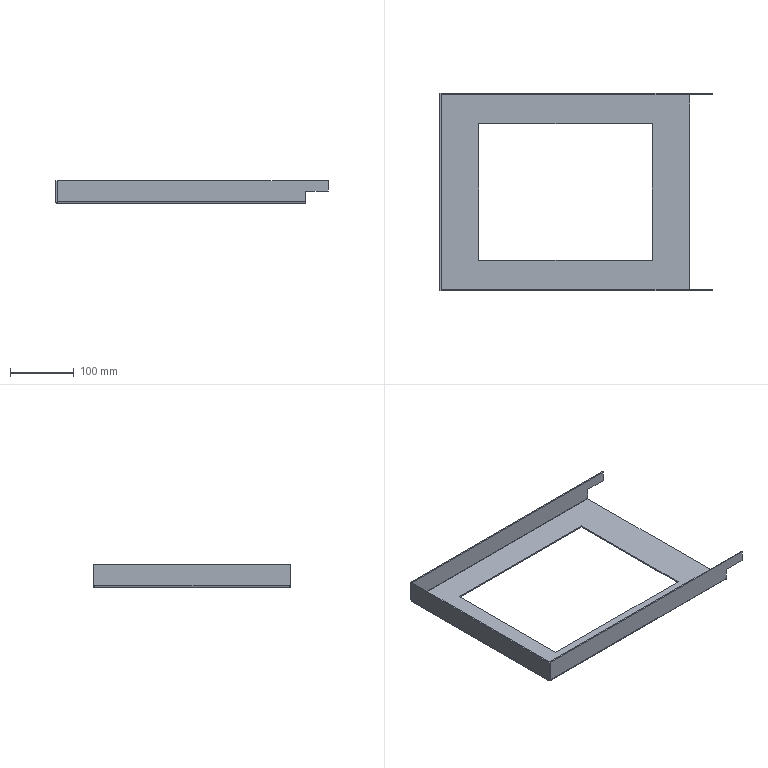Part | SolidWorks | features BaseBody 1 | 1 solid | 40 faces | box 428 x 310 x 36 mm | volume 201770 mm3 | plane 34 | cylinder 6 | commonest cylinder face diameters 1 x3 5 x3
STEP:
#1=CARTESIAN_POINT('',(196.5,-155.,17.5));
#2=VERTEX_POINT('',#1);
#3=CARTESIAN_POINT('',(231.5,-155.,17.5));
#4=VERTEX_POINT('',#3);
#5=CARTESIAN_POINT('',(196.5,-155.,17.5));
#6=DIRECTION('',(1.,0.,0.));
#7=VECTOR('',#6,1000.);
#8=LINE('',#5,#7);
#9=EDGE_CURVE('',#2,#4,#8,.T.);
#10=ORIENTED_EDGE('',*,*,#9,.F.);
#11=CARTESIAN_POINT('',(196.5,-153.,17.5));
#12=VERTEX_POINT('',#11);
#13=CARTESIAN_POINT('',(196.5,-153.,17.5));
#14=DIRECTION('',(0.,-1.,0.));
#15=VECTOR('',#14,1000.);
#16=LINE('',#13,#15);
#17=EDGE_CURVE('',#12,#2,#16,.T.);
#18=ORIENTED_EDGE('',*,*,#17,.F.);
#19=CARTESIAN_POINT('',(231.5,-153.,17.5));
#20=VERTEX_POINT('',#19);
#21=CARTESIAN_POINT('',(196.5,-153.,17.5));
#22=DIRECTION('',(1.,0.,0.));
#23=VECTOR('',#22,1000.);
#24=LINE('',#21,#23);
#25=EDGE_CURVE('',#12,#20,#24,.T.);
#26=ORIENTED_EDGE('',*,*,#25,.T.);
#27=CARTESIAN_POINT('',(231.5,-153.,17.5));
#28=DIRECTION('',(0.,-1.,0.));
#29=VECTOR('',#28,1000.);
#30=LINE('',#27,#29);
#31=EDGE_CURVE('',#20,#4,#30,.T.);
#32=ORIENTED_EDGE('',*,*,#31,.T.);
#33=EDGE_LOOP('',(#10,#18,#26,#32));
#34=FACE_OUTER_BOUND('',#33,.T.);
#35=CARTESIAN_POINT('',(196.5,-153.,17.5));
#36=DIRECTION('',(0.,0.,-1.));
#37=DIRECTION('',(-1.,0.,0.));
#38=AXIS2_PLACEMENT_3D('',#35,#36,#37);
#39=PLANE('',#38);
#40=ADVANCED_FACE('',(#34),#39,.T.);
#41=CARTESIAN_POINT('',(231.5,-155.,34.));
#42=VERTEX_POINT('',#41);
#43=CARTESIAN_POINT('',(231.5,-155.,34.));
#44=DIRECTION('',(0.,0.,1.));
#45=VECTOR('',#44,1000.);
#46=LINE('',#43,#45);
#47=EDGE_CURVE('',#4,#42,#46,.T.);
#48=ORIENTED_EDGE('',*,*,#47,.F.);
#49=ORIENTED_EDGE('',*,*,#31,.F.);
#50=CARTESIAN_POINT('',(231.5,-153.,34.));
#51=VERTEX_POINT('',#50);
#52=CARTESIAN_POINT('',(231.5,-153.,34.));
#53=DIRECTION('',(0.,0.,1.));
#54=VECTOR('',#53,1000.);
#55=LINE('',#52,#54);
#56=EDGE_CURVE('',#20,#51,#55,.T.);
#57=ORIENTED_EDGE('',*,*,#56,.T.);
#58=CARTESIAN_POINT('',(231.5,-153.,34.));
#59=DIRECTION('',(0.,-1.,0.));
#60=VECTOR('',#59,1000.);
#61=LINE('',#58,#60);
#62=EDGE_CURVE('',#51,#42,#61,.T.);
#63=ORIENTED_EDGE('',*,*,#62,.T.);
#64=EDGE_LOOP('',(#48,#49,#57,#63));
#65=FACE_OUTER_BOUND('',#64,.T.);
#66=CARTESIAN_POINT('',(231.5,-153.,34.));
#67=DIRECTION('',(1.,0.,0.));
#68=DIRECTION('',(0.,1.,0.));
#69=AXIS2_PLACEMENT_3D('',#66,#67,#68);
#70=PLANE('',#69);
#71=ADVANCED_FACE('',(#65),#70,.T.);
#72=CARTESIAN_POINT('',(137.,-107.5,-2.));
#73=VERTEX_POINT('',#72);
#74=CARTESIAN_POINT('',(-135.,-107.5,-2.));
#75=VERTEX_POINT('',#74);
#76=CARTESIAN_POINT('',(-135.,-107.5,-2.));
#77=DIRECTION('',(-1.,0.,0.));
#78=VECTOR('',#77,1000.);
#79=LINE('',#76,#78);
#80=EDGE_CURVE('',#73,#75,#79,.T.);
#81=ORIENTED_EDGE('',*,*,#80,.T.);
#82=CARTESIAN_POINT('',(-135.,-107.5,0.));
#83=VERTEX_POINT('',#82);
#84=CARTESIAN_POINT('',(-135.,-107.5,0.));
#85=DIRECTION('',(0.,0.,-1.));
#86=VECTOR('',#85,1000.);
#87=LINE('',#84,#86);
#88=EDGE_CURVE('',#83,#75,#87,.T.);
#89=ORIENTED_EDGE('',*,*,#88,.F.);
#90=CARTESIAN_POINT('',(137.,-107.5,0.));
#91=VERTEX_POINT('',#90);
#92=CARTESIAN_POINT('',(-135.,-107.5,0.));
#93=DIRECTION('',(-1.,0.,0.));
#94=VECTOR('',#93,1000.);
#95=LINE('',#92,#94);
#96=EDGE_CURVE('',#91,#83,#95,.T.);
#97=ORIENTED_EDGE('',*,*,#96,.F.);
#98=CARTESIAN_POINT('',(137.,-107.5,0.));
#99=DIRECTION('',(0.,0.,-1.));
#100=VECTOR('',#99,1000.);
#101=LINE('',#98,#100);
#102=EDGE_CURVE('',#91,#73,#101,.T.);
#103=ORIENTED_EDGE('',*,*,#102,.T.);
#104=EDGE_LOOP('',(#81,#89,#97,#103));
#105=FACE_OUTER_BOUND('',#104,.T.);
#106=CARTESIAN_POINT('',(-135.,-107.5,0.));
#107=DIRECTION('',(0.,-1.,0.));
#108=DIRECTION('',(-1.,0.,0.));
#109=AXIS2_PLACEMENT_3D('',#106,#107,#108);
#110=PLANE('',#109);
#111=ADVANCED_FACE('',(#105),#110,.F.);
#112=CARTESIAN_POINT('',(-135.,107.5,-2.));
#113=VERTEX_POINT('',#112);
#114=CARTESIAN_POINT('',(-135.,107.5,-2.));
#115=DIRECTION('',(0.,1.,0.));
#116=VECTOR('',#115,1000.);
#117=LINE('',#114,#116);
#118=EDGE_CURVE('',#75,#113,#117,.T.);
#119=ORIENTED_EDGE('',*,*,#118,.T.);
#120=CARTESIAN_POINT('',(-135.,107.5,0.));
#121=VERTEX_POINT('',#120);
#122=CARTESIAN_POINT('',(-135.,107.5,0.));
#123=DIRECTION('',(0.,0.,-1.));
#124=VECTOR('',#123,1000.);
#125=LINE('',#122,#124);
#126=EDGE_CURVE('',#121,#113,#125,.T.);
#127=ORIENTED_EDGE('',*,*,#126,.F.);
#128=CARTESIAN_POINT('',(-135.,107.5,0.));
#129=DIRECTION('',(0.,1.,0.));
#130=VECTOR('',#129,1000.);
#131=LINE('',#128,#130);
#132=EDGE_CURVE('',#83,#121,#131,.T.);
#133=ORIENTED_EDGE('',*,*,#132,.F.);
#134=ORIENTED_EDGE('',*,*,#88,.T.);
#135=EDGE_LOOP('',(#119,#127,#133,#134));
#136=FACE_OUTER_BOUND('',#135,.T.);
#137=CARTESIAN_POINT('',(-135.,107.5,0.));
#138=DIRECTION('',(-1.,0.,0.));
#139=DIRECTION('',(0.,0.,1.));
#140=AXIS2_PLACEMENT_3D('',#137,#138,#139);
#141=PLANE('',#140);
#142=ADVANCED_FACE('',(#136),#141,.F.);
#143=CARTESIAN_POINT('',(137.,107.5,-2.));
#144=VERTEX_POINT('',#143);
#145=CARTESIAN_POINT('',(-135.,107.5,-2.));
#146=DIRECTION('',(1.,0.,0.));
#147=VECTOR('',#146,1000.);
#148=LINE('',#145,#147);
#149=EDGE_CURVE('',#113,#144,#148,.T.);
#150=ORIENTED_EDGE('',*,*,#149,.T.);
#151=CARTESIAN_POINT('',(137.,107.5,0.));
#152=VERTEX_POINT('',#151);
#153=CARTESIAN_POINT('',(137.,107.5,0.));
#154=DIRECTION('',(0.,0.,-1.));
#155=VECTOR('',#154,1000.);
#156=LINE('',#153,#155);
#157=EDGE_CURVE('',#152,#144,#156,.T.);
#158=ORIENTED_EDGE('',*,*,#157,.F.);
#159=CARTESIAN_POINT('',(-135.,107.5,0.));
#160=DIRECTION('',(1.,0.,0.));
#161=VECTOR('',#160,1000.);
#162=LINE('',#159,#161);
#163=EDGE_CURVE('',#121,#152,#162,.T.);
#164=ORIENTED_EDGE('',*,*,#163,.F.);
#165=ORIENTED_EDGE('',*,*,#126,.T.);
#166=EDGE_LOOP('',(#150,#158,#164,#165));
#167=FACE_OUTER_BOUND('',#166,.T.);
#168=CARTESIAN_POINT('',(-135.,107.5,0.));
#169=DIRECTION('',(0.,1.,0.));
#170=DIRECTION('',(1.,0.,0.));
#171=AXIS2_PLACEMENT_3D('',#168,#169,#170);
#172=PLANE('',#171);
#173=ADVANCED_FACE('',(#167),#172,.F.);
#174=CARTESIAN_POINT('',(137.,107.5,-2.));
#175=DIRECTION('',(0.,-1.,0.));
#176=VECTOR('',#175,1000.);
#177=LINE('',#174,#176);
#178=EDGE_CURVE('',#144,#73,#177,.T.);
#179=ORIENTED_EDGE('',*,*,#178,.T.);
#180=ORIENTED_EDGE('',*,*,#102,.F.);
#181=CARTESIAN_POINT('',(137.,107.5,0.));
#182=DIRECTION('',(0.,-1.,0.));
#183=VECTOR('',#182,1000.);
#184=LINE('',#181,#183);
#185=EDGE_CURVE('',#152,#91,#184,.T.);
#186=ORIENTED_EDGE('',*,*,#185,.F.);
#187=ORIENTED_EDGE('',*,*,#157,.T.);
#188=EDGE_LOOP('',(#179,#180,#186,#187));
#189=FACE_OUTER_BOUND('',#188,.T.);
#190=CARTESIAN_POINT('',(137.,107.5,0.));
#191=DIRECTION('',(1.,0.,0.));
#192=DIRECTION('',(0.,-1.,0.));
#193=AXIS2_PLACEMENT_3D('',#190,#191,#192);
#194=PLANE('',#193);
#195=ADVANCED_FACE('',(#189),#194,.F.);
#196=CARTESIAN_POINT('',(231.5,155.,34.));
#197=VERTEX_POINT('',#196);
#198=CARTESIAN_POINT('',(231.5,155.,17.5));
#199=VERTEX_POINT('',#198);
#200=CARTESIAN_POINT('',(231.5,155.,34.));
#201=DIRECTION('',(0.,0.,-1.));
#202=VECTOR('',#201,1000.);
#203=LINE('',#200,#202);
#204=EDGE_CURVE('',#197,#199,#203,.T.);
#205=ORIENTED_EDGE('',*,*,#204,.F.);
#206=CARTESIAN_POINT('',(231.5,153.,34.));
#207=VERTEX_POINT('',#206);
#208=CARTESIAN_POINT('',(231.5,153.,34.));
#209=DIRECTION('',(0.,1.,0.));
#210=VECTOR('',#209,1000.);
#211=LINE('',#208,#210);
#212=EDGE_CURVE('',#207,#197,#211,.T.);
#213=ORIENTED_EDGE('',*,*,#212,.F.);
#214=CARTESIAN_POINT('',(231.5,153.,17.5));
#215=VERTEX_POINT('',#214);
#216=CARTESIAN_POINT('',(231.5,153.,34.));
#217=DIRECTION('',(0.,0.,-1.));
#218=VECTOR('',#217,1000.);
#219=LINE('',#216,#218);
#220=EDGE_CURVE('',#207,#215,#219,.T.);
#221=ORIENTED_EDGE('',*,*,#220,.T.);
#222=CARTESIAN_POINT('',(231.5,153.,17.5));
#223=DIRECTION('',(0.,1.,0.));
#224=VECTOR('',#223,1000.);
#225=LINE('',#222,#224);
#226=EDGE_CURVE('',#215,#199,#225,.T.);
#227=ORIENTED_EDGE('',*,*,#226,.T.);
#228=EDGE_LOOP('',(#205,#213,#221,#227));
#229=FACE_OUTER_BOUND('',#228,.T.);
#230=CARTESIAN_POINT('',(231.5,153.,34.));
#231=DIRECTION('',(1.,0.,0.));
#232=DIRECTION('',(0.,1.,0.));
#233=AXIS2_PLACEMENT_3D('',#230,#231,#232);
#234=PLANE('',#233);
#235=ADVANCED_FACE('',(#229),#234,.T.);
#236=CARTESIAN_POINT('',(196.5,155.,17.5));
#237=VERTEX_POINT('',#236);
#238=CARTESIAN_POINT('',(196.5,155.,17.5));
#239=DIRECTION('',(-1.,0.,0.));
#240=VECTOR('',#239,1000.);
#241=LINE('',#238,#240);
#242=EDGE_CURVE('',#199,#237,#241,.T.);
#243=ORIENTED_EDGE('',*,*,#242,.F.);
#244=ORIENTED_EDGE('',*,*,#226,.F.);
#245=CARTESIAN_POINT('',(196.5,153.,17.5));
#246=VERTEX_POINT('',#245);
#247=CARTESIAN_POINT('',(196.5,153.,17.5));
#248=DIRECTION('',(-1.,0.,0.));
#249=VECTOR('',#248,1000.);
#250=LINE('',#247,#249);
#251=EDGE_CURVE('',#215,#246,#250,.T.);
#252=ORIENTED_EDGE('',*,*,#251,.T.);
#253=CARTESIAN_POINT('',(196.5,153.,17.5));
#254=DIRECTION('',(0.,1.,0.));
#255=VECTOR('',#254,1000.);
#256=LINE('',#253,#255);
#257=EDGE_CURVE('',#246,#237,#256,.T.);
#258=ORIENTED_EDGE('',*,*,#257,.T.);
#259=EDGE_LOOP('',(#243,#244,#252,#258));
#260=FACE_OUTER_BOUND('',#259,.T.);
#261=CARTESIAN_POINT('',(196.5,153.,17.5));
#262=DIRECTION('',(0.,0.,-1.));
#263=DIRECTION('',(0.,-1.,0.));
#264=AXIS2_PLACEMENT_3D('',#261,#262,#263);
#265=PLANE('',#264);
#266=ADVANCED_FACE('',(#260),#265,.T.);
#267=CARTESIAN_POINT('',(-194.,-153.,34.));
#268=VERTEX_POINT('',#267);
#269=CARTESIAN_POINT('',(-194.,-153.,34.));
#270=DIRECTION('',(-1.,0.,0.));
#271=VECTOR('',#270,1000.);
#272=LINE('',#269,#271);
#273=EDGE_CURVE('',#51,#268,#272,.T.);
#274=ORIENTED_EDGE('',*,*,#273,.T.);
#275=CARTESIAN_POINT('',(-194.,-155.,34.));
#276=VERTEX_POINT('',#275);
#277=CARTESIAN_POINT('',(-194.,-155.,34.));
#278=DIRECTION('',(0.,1.,0.));
#279=VECTOR('',#278,1000.);
#280=LINE('',#277,#279);
#281=EDGE_CURVE('',#276,#268,#280,.T.);
#282=ORIENTED_EDGE('',*,*,#281,.F.);
#283=CARTESIAN_POINT('',(0.,-155.,34.));
#284=DIRECTION('',(-1.,0.,0.));
#285=VECTOR('',#284,1000.);
#286=LINE('',#283,#285);
#287=EDGE_CURVE('',#42,#276,#286,.T.);
#288=ORIENTED_EDGE('',*,*,#287,.F.);
#289=ORIENTED_EDGE('',*,*,#62,.F.);
#290=EDGE_LOOP('',(#274,#282,#288,#289));
#291=FACE_OUTER_BOUND('',#290,.T.);
#292=CARTESIAN_POINT('',(-194.,-155.,34.));
#293=DIRECTION('',(0.,0.,-1.));
#294=DIRECTION('',(-1.,0.,0.));
#295=AXIS2_PLACEMENT_3D('',#292,#293,#294);
#296=PLANE('',#295);
#297=ADVANCED_FACE('',(#291),#296,.F.);
#298=CARTESIAN_POINT('',(196.5,-153.,0.5));
#299=VERTEX_POINT('',#298);
#300=CARTESIAN_POINT('',(196.5,-153.,34.));
#301=DIRECTION('',(0.,0.,1.));
#302=VECTOR('',#301,1000.);
#303=LINE('',#300,#302);
#304=EDGE_CURVE('',#299,#12,#303,.T.);
#305=ORIENTED_EDGE('',*,*,#304,.F.);
#306=CARTESIAN_POINT('',(-194.,-153.,0.5));
#307=VERTEX_POINT('',#306);
#308=CARTESIAN_POINT('',(-194.,-153.,0.5));
#309=DIRECTION('',(1.,0.,0.));
#310=VECTOR('',#309,1000.);
#311=LINE('',#308,#310);
#312=EDGE_CURVE('',#307,#299,#311,.T.);
#313=ORIENTED_EDGE('',*,*,#312,.F.);
#314=CARTESIAN_POINT('',(-194.,-153.,0.));
#315=DIRECTION('',(0.,0.,-1.));
#316=VECTOR('',#315,1000.);
#317=LINE('',#314,#316);
#318=EDGE_CURVE('',#268,#307,#317,.T.);
#319=ORIENTED_EDGE('',*,*,#318,.F.);
#320=ORIENTED_EDGE('',*,*,#273,.F.);
#321=ORIENTED_EDGE('',*,*,#56,.F.);
#322=ORIENTED_EDGE('',*,*,#25,.F.);
#323=EDGE_LOOP('',(#305,#313,#319,#320,#321,#322));
#324=FACE_OUTER_BOUND('',#323,.T.);
#325=CARTESIAN_POINT('',(0.,-153.,0.));
#326=DIRECTION('',(0.,1.,0.));
#327=DIRECTION('',(0.,0.,-1.));
#328=AXIS2_PLACEMENT_3D('',#325,#326,#327);
#329=PLANE('',#328);
#330=ADVANCED_FACE('',(#324),#329,.T.);
#331=CARTESIAN_POINT('',(196.5,-155.,0.5));
#332=VERTEX_POINT('',#331);
#333=CARTESIAN_POINT('',(-194.,-155.,0.5));
#334=VERTEX_POINT('',#333);
#335=CARTESIAN_POINT('',(-194.,-155.,0.5));
#336=DIRECTION('',(-1.,0.,0.));
#337=VECTOR('',#336,1000.);
#338=LINE('',#335,#337);
#339=EDGE_CURVE('',#332,#334,#338,.T.);
#340=ORIENTED_EDGE('',*,*,#339,.F.);
#341=CARTESIAN_POINT('',(196.5,-155.,0.));
#342=DIRECTION('',(0.,0.,1.));
#343=VECTOR('',#342,1000.);
#344=LINE('',#341,#343);
#345=EDGE_CURVE('',#332,#2,#344,.T.);
#346=ORIENTED_EDGE('',*,*,#345,.T.);
#347=ORIENTED_EDGE('',*,*,#9,.T.);
#348=ORIENTED_EDGE('',*,*,#47,.T.);
#349=ORIENTED_EDGE('',*,*,#287,.T.);
#350=CARTESIAN_POINT('',(-194.,-155.,0.));
#351=DIRECTION('',(0.,0.,-1.));
#352=VECTOR('',#351,1000.);
#353=LINE('',#350,#352);
#354=EDGE_CURVE('',#276,#334,#353,.T.);
#355=ORIENTED_EDGE('',*,*,#354,.T.);
#356=EDGE_LOOP('',(#340,#346,#347,#348,#349,#355));
#357=FACE_OUTER_BOUND('',#356,.T.);
#358=CARTESIAN_POINT('',(0.,-155.,0.));
#359=DIRECTION('',(0.,1.,0.));
#360=DIRECTION('',(0.,0.,-1.));
#361=AXIS2_PLACEMENT_3D('',#358,#359,#360);
#362=PLANE('',#361);
#363=ADVANCED_FACE('',(#357),#362,.F.);
#364=CARTESIAN_POINT('',(-194.,-155.,0.5));
#365=DIRECTION('',(0.,-1.,0.));
#366=VECTOR('',#365,1000.);
#367=LINE('',#364,#366);
#368=EDGE_CURVE('',#307,#334,#367,.T.);
#369=ORIENTED_EDGE('',*,*,#368,.T.);
#370=ORIENTED_EDGE('',*,*,#354,.F.);
#371=ORIENTED_EDGE('',*,*,#281,.T.);
#372=ORIENTED_EDGE('',*,*,#318,.T.);
#373=EDGE_LOOP('',(#369,#370,#371,#372));
#374=FACE_OUTER_BOUND('',#373,.T.);
#375=CARTESIAN_POINT('',(-194.,-155.,0.));
#376=DIRECTION('',(1.,0.,0.));
#377=DIRECTION('',(0.,1.,0.));
#378=AXIS2_PLACEMENT_3D('',#375,#376,#377);
#379=PLANE('',#378);
#380=ADVANCED_FACE('',(#374),#379,.F.);
#381=ORIENTED_EDGE('',*,*,#304,.T.);
#382=ORIENTED_EDGE('',*,*,#17,.T.);
#383=ORIENTED_EDGE('',*,*,#345,.F.);
#384=CARTESIAN_POINT('',(196.5,-153.,0.5));
#385=DIRECTION('',(0.,-1.,0.));
#386=VECTOR('',#385,1000.);
#387=LINE('',#384,#386);
#388=EDGE_CURVE('',#299,#332,#387,.T.);
#389=ORIENTED_EDGE('',*,*,#388,.F.);
#390=EDGE_LOOP('',(#381,#382,#383,#389));
#391=FACE_OUTER_BOUND('',#390,.T.);
#392=CARTESIAN_POINT('',(196.5,-155.,34.));
#393=DIRECTION('',(-1.,0.,0.));
#394=DIRECTION('',(0.,1.,0.));
#395=AXIS2_PLACEMENT_3D('',#392,#393,#394);
#396=PLANE('',#395);
#397=ADVANCED_FACE('',(#391),#396,.F.);
#398=CARTESIAN_POINT('',(196.5,-152.5,0.));
#399=VERTEX_POINT('',#398);
#400=CARTESIAN_POINT('',(-194.,-152.5,0.));
#401=VERTEX_POINT('',#400);
#402=CARTESIAN_POINT('',(196.5,-152.5,0.));
#403=DIRECTION('',(-1.,0.,0.));
#404=VECTOR('',#403,1000.);
#405=LINE('',#402,#404);
#406=EDGE_CURVE('',#399,#401,#405,.T.);
#407=ORIENTED_EDGE('',*,*,#406,.T.);
#408=CARTESIAN_POINT('',(-194.,-152.5,0.5));
#409=DIRECTION('',(-1.,0.,0.));
#410=DIRECTION('',(0.,0.,-1.));
#411=AXIS2_PLACEMENT_3D('',#408,#409,#410);
#412=CIRCLE('',#411,0.5);
#413=EDGE_CURVE('',#401,#307,#412,.T.);
#414=ORIENTED_EDGE('',*,*,#413,.T.);
#415=ORIENTED_EDGE('',*,*,#312,.T.);
#416=CARTESIAN_POINT('',(196.5,-152.5,0.5));
#417=DIRECTION('',(1.,0.,0.));
#418=DIRECTION('',(0.,0.,-1.));
#419=AXIS2_PLACEMENT_3D('',#416,#417,#418);
#420=CIRCLE('',#419,0.5);
#421=EDGE_CURVE('',#299,#399,#420,.T.);
#422=ORIENTED_EDGE('',*,*,#421,.T.);
#423=EDGE_LOOP('',(#407,#414,#415,#422));
#424=FACE_OUTER_BOUND('',#423,.T.);
#425=CARTESIAN_POINT('',(196.5,-152.5,0.5));
#426=DIRECTION('',(1.,0.,0.));
#427=DIRECTION('',(0.,-1.,0.));
#428=AXIS2_PLACEMENT_3D('',#425,#426,#427);
#429=CYLINDRICAL_SURFACE('',#428,0.5);
#430=ADVANCED_FACE('',(#424),#429,.F.);
#431=CARTESIAN_POINT('',(196.5,-152.5,-2.));
#432=VERTEX_POINT('',#431);
#433=CARTESIAN_POINT('',(-194.,-152.5,-2.));
#434=VERTEX_POINT('',#433);
#435=CARTESIAN_POINT('',(196.5,-152.5,-2.));
#436=DIRECTION('',(-1.,0.,0.));
#437=VECTOR('',#436,1000.);
#438=LINE('',#435,#437);
#439=EDGE_CURVE('',#432,#434,#438,.T.);
#440=ORIENTED_EDGE('',*,*,#439,.F.);
#441=CARTESIAN_POINT('',(196.5,-152.5,0.5));
#442=DIRECTION('',(1.,0.,0.));
#443=DIRECTION('',(0.,0.,-1.));
#444=AXIS2_PLACEMENT_3D('',#441,#442,#443);
#445=CIRCLE('',#444,2.5);
#446=EDGE_CURVE('',#332,#432,#445,.T.);
#447=ORIENTED_EDGE('',*,*,#446,.F.);
#448=ORIENTED_EDGE('',*,*,#339,.T.);
#449=CARTESIAN_POINT('',(-194.,-152.5,0.5));
#450=DIRECTION('',(-1.,0.,0.));
#451=DIRECTION('',(0.,0.,-1.));
#452=AXIS2_PLACEMENT_3D('',#449,#450,#451);
#453=CIRCLE('',#452,2.5);
#454=EDGE_CURVE('',#434,#334,#453,.T.);
#455=ORIENTED_EDGE('',*,*,#454,.F.);
#456=EDGE_LOOP('',(#440,#447,#448,#455));
#457=FACE_OUTER_BOUND('',#456,.T.);
#458=CARTESIAN_POINT('',(196.5,-152.5,0.5));
#459=DIRECTION('',(1.,0.,0.));
#460=DIRECTION('',(0.,-1.,0.));
#461=AXIS2_PLACEMENT_3D('',#458,#459,#460);
#462=CYLINDRICAL_SURFACE('',#461,2.5);
#463=ADVANCED_FACE('',(#457),#462,.T.);
#464=ORIENTED_EDGE('',*,*,#421,.F.);
#465=ORIENTED_EDGE('',*,*,#388,.T.);
#466=ORIENTED_EDGE('',*,*,#446,.T.);
#467=CARTESIAN_POINT('',(196.5,-152.5,0.));
#468=DIRECTION('',(0.,0.,-1.));
#469=VECTOR('',#468,1000.);
#470=LINE('',#467,#469);
#471=EDGE_CURVE('',#399,#432,#470,.T.);
#472=ORIENTED_EDGE('',*,*,#471,.F.);
#473=EDGE_LOOP('',(#464,#465,#466,#472));
#474=FACE_OUTER_BOUND('',#473,.T.);
#475=CARTESIAN_POINT('',(196.5,-152.5,0.5));
#476=DIRECTION('',(-1.,0.,0.));
#477=DIRECTION('',(0.,1.,0.));
#478=AXIS2_PLACEMENT_3D('',#475,#476,#477);
#479=PLANE('',#478);
#480=ADVANCED_FACE('',(#474),#479,.F.);
#481=ORIENTED_EDGE('',*,*,#368,.F.);
#482=ORIENTED_EDGE('',*,*,#413,.F.);
#483=CARTESIAN_POINT('',(-194.,-152.5,0.));
#484=DIRECTION('',(0.,0.,-1.));
#485=VECTOR('',#484,1000.);
#486=LINE('',#483,#485);
#487=EDGE_CURVE('',#401,#434,#486,.T.);
#488=ORIENTED_EDGE('',*,*,#487,.T.);
#489=ORIENTED_EDGE('',*,*,#454,.T.);
#490=EDGE_LOOP('',(#481,#482,#488,#489));
#491=FACE_OUTER_BOUND('',#490,.T.);
#492=CARTESIAN_POINT('',(-194.,-152.5,0.5));
#493=DIRECTION('',(-1.,0.,0.));
#494=DIRECTION('',(0.,1.,0.));
#495=AXIS2_PLACEMENT_3D('',#492,#493,#494);
#496=PLANE('',#495);
#497=ADVANCED_FACE('',(#491),#496,.T.);
#498=CARTESIAN_POINT('',(-194.,153.,34.));
#499=VERTEX_POINT('',#498);
#500=CARTESIAN_POINT('',(196.5,153.,34.));
#501=DIRECTION('',(1.,0.,0.));
#502=VECTOR('',#501,1000.);
#503=LINE('',#500,#502);
#504=EDGE_CURVE('',#499,#207,#503,.T.);
#505=ORIENTED_EDGE('',*,*,#504,.T.);
#506=ORIENTED_EDGE('',*,*,#212,.T.);
#507=CARTESIAN_POINT('',(-194.,155.,34.));
#508=VERTEX_POINT('',#507);
#509=CARTESIAN_POINT('',(0.,155.,34.));
#510=DIRECTION('',(1.,0.,0.));
#511=VECTOR('',#510,1000.);
#512=LINE('',#509,#511);
#513=EDGE_CURVE('',#508,#197,#512,.T.);
#514=ORIENTED_EDGE('',*,*,#513,.F.);
#515=CARTESIAN_POINT('',(-194.,155.,34.));
#516=DIRECTION('',(0.,-1.,0.));
#517=VECTOR('',#516,1000.);
#518=LINE('',#515,#517);
#519=EDGE_CURVE('',#508,#499,#518,.T.);
#520=ORIENTED_EDGE('',*,*,#519,.T.);
#521=EDGE_LOOP('',(#505,#506,#514,#520));
#522=FACE_OUTER_BOUND('',#521,.T.);
#523=CARTESIAN_POINT('',(196.5,155.,34.));
#524=DIRECTION('',(0.,0.,-1.));
#525=DIRECTION('',(0.,-1.,0.));
#526=AXIS2_PLACEMENT_3D('',#523,#524,#525);
#527=PLANE('',#526);
#528=ADVANCED_FACE('',(#522),#527,.F.);
#529=CARTESIAN_POINT('',(-194.,153.,0.5));
#530=VERTEX_POINT('',#529);
#531=CARTESIAN_POINT('',(-194.,153.,34.));
#532=DIRECTION('',(0.,0.,1.));
#533=VECTOR('',#532,1000.);
#534=LINE('',#531,#533);
#535=EDGE_CURVE('',#530,#499,#534,.T.);
#536=ORIENTED_EDGE('',*,*,#535,.F.);
#537=CARTESIAN_POINT('',(196.5,153.,0.5));
#538=VERTEX_POINT('',#537);
#539=CARTESIAN_POINT('',(196.5,153.,0.5));
#540=DIRECTION('',(-1.,0.,0.));
#541=VECTOR('',#540,1000.);
#542=LINE('',#539,#541);
#543=EDGE_CURVE('',#538,#530,#542,.T.);
#544=ORIENTED_EDGE('',*,*,#543,.F.);
#545=CARTESIAN_POINT('',(196.5,153.,0.));
#546=DIRECTION('',(0.,0.,-1.));
#547=VECTOR('',#546,1000.);
#548=LINE('',#545,#547);
#549=EDGE_CURVE('',#246,#538,#548,.T.);
#550=ORIENTED_EDGE('',*,*,#549,.F.);
#551=ORIENTED_EDGE('',*,*,#251,.F.);
#552=ORIENTED_EDGE('',*,*,#220,.F.);
#553=ORIENTED_EDGE('',*,*,#504,.F.);
#554=EDGE_LOOP('',(#536,#544,#550,#551,#552,#553));
#555=FACE_OUTER_BOUND('',#554,.T.);
#556=CARTESIAN_POINT('',(0.,153.,0.));
#557=DIRECTION('',(0.,-1.,0.));
#558=DIRECTION('',(-1.,0.,0.));
#559=AXIS2_PLACEMENT_3D('',#556,#557,#558);
#560=PLANE('',#559);
#561=ADVANCED_FACE('',(#555),#560,.T.);
#562=CARTESIAN_POINT('',(-194.,155.,0.5));
#563=VERTEX_POINT('',#562);
#564=CARTESIAN_POINT('',(196.5,155.,0.5));
#565=VERTEX_POINT('',#564);
#566=CARTESIAN_POINT('',(196.5,155.,0.5));
#567=DIRECTION('',(1.,0.,0.));
#568=VECTOR('',#567,1000.);
#569=LINE('',#566,#568);
#570=EDGE_CURVE('',#563,#565,#569,.T.);
#571=ORIENTED_EDGE('',*,*,#570,.F.);
#572=CARTESIAN_POINT('',(-194.,155.,0.));
#573=DIRECTION('',(0.,0.,1.));
#574=VECTOR('',#573,1000.);
#575=LINE('',#572,#574);
#576=EDGE_CURVE('',#563,#508,#575,.T.);
#577=ORIENTED_EDGE('',*,*,#576,.T.);
#578=ORIENTED_EDGE('',*,*,#513,.T.);
#579=ORIENTED_EDGE('',*,*,#204,.T.);
#580=ORIENTED_EDGE('',*,*,#242,.T.);
#581=CARTESIAN_POINT('',(196.5,155.,0.));
#582=DIRECTION('',(0.,0.,-1.));
#583=VECTOR('',#582,1000.);
#584=LINE('',#581,#583);
#585=EDGE_CURVE('',#237,#565,#584,.T.);
#586=ORIENTED_EDGE('',*,*,#585,.T.);
#587=EDGE_LOOP('',(#571,#577,#578,#579,#580,#586));
#588=FACE_OUTER_BOUND('',#587,.T.);
#589=CARTESIAN_POINT('',(0.,155.,0.));
#590=DIRECTION('',(0.,-1.,0.));
#591=DIRECTION('',(-1.,0.,0.));
#592=AXIS2_PLACEMENT_3D('',#589,#590,#591);
#593=PLANE('',#592);
#594=ADVANCED_FACE('',(#588),#593,.F.);
#595=CARTESIAN_POINT('',(-194.,153.,0.5));
#596=DIRECTION('',(0.,1.,0.));
#597=VECTOR('',#596,1000.);
#598=LINE('',#595,#597);
#599=EDGE_CURVE('',#530,#563,#598,.T.);
#600=ORIENTED_EDGE('',*,*,#599,.F.);
#601=ORIENTED_EDGE('',*,*,#535,.T.);
#602=ORIENTED_EDGE('',*,*,#519,.F.);
#603=ORIENTED_EDGE('',*,*,#576,.F.);
#604=EDGE_LOOP('',(#600,#601,#602,#603));
#605=FACE_OUTER_BOUND('',#604,.T.);
#606=CARTESIAN_POINT('',(-194.,155.,34.));
#607=DIRECTION('',(1.,0.,0.));
#608=DIRECTION('',(0.,1.,0.));
#609=AXIS2_PLACEMENT_3D('',#606,#607,#608);
#610=PLANE('',#609);
#611=ADVANCED_FACE('',(#605),#610,.F.);
#612=ORIENTED_EDGE('',*,*,#585,.F.);
#613=ORIENTED_EDGE('',*,*,#257,.F.);
#614=ORIENTED_EDGE('',*,*,#549,.T.);
#615=CARTESIAN_POINT('',(196.5,155.,0.5));
#616=DIRECTION('',(0.,1.,0.));
#617=VECTOR('',#616,1000.);
#618=LINE('',#615,#617);
#619=EDGE_CURVE('',#538,#565,#618,.T.);
#620=ORIENTED_EDGE('',*,*,#619,.T.);
#621=EDGE_LOOP('',(#612,#613,#614,#620));
#622=FACE_OUTER_BOUND('',#621,.T.);
#623=CARTESIAN_POINT('',(196.5,155.,0.));
#624=DIRECTION('',(-1.,0.,0.));
#625=DIRECTION('',(0.,1.,0.));
#626=AXIS2_PLACEMENT_3D('',#623,#624,#625);
#627=PLANE('',#626);
#628=ADVANCED_FACE('',(#622),#627,.F.);
#629=CARTESIAN_POINT('',(-194.,152.5,0.));
#630=VERTEX_POINT('',#629);
#631=CARTESIAN_POINT('',(196.5,152.5,0.));
#632=VERTEX_POINT('',#631);
#633=CARTESIAN_POINT('',(-194.,152.5,0.));
#634=DIRECTION('',(1.,0.,0.));
#635=VECTOR('',#634,1000.);
#636=LINE('',#633,#635);
#637=EDGE_CURVE('',#630,#632,#636,.T.);
#638=ORIENTED_EDGE('',*,*,#637,.T.);
#639=CARTESIAN_POINT('',(196.5,152.5,0.5));
#640=DIRECTION('',(1.,0.,0.));
#641=DIRECTION('',(0.,0.,1.));
#642=AXIS2_PLACEMENT_3D('',#639,#640,#641);
#643=CIRCLE('',#642,0.5);
#644=EDGE_CURVE('',#632,#538,#643,.T.);
#645=ORIENTED_EDGE('',*,*,#644,.T.);
#646=ORIENTED_EDGE('',*,*,#543,.T.);
#647=CARTESIAN_POINT('',(-194.,152.5,0.5));
#648=DIRECTION('',(-1.,0.,0.));
#649=DIRECTION('',(0.,0.,1.));
#650=AXIS2_PLACEMENT_3D('',#647,#648,#649);
#651=CIRCLE('',#650,0.5);
#652=EDGE_CURVE('',#530,#630,#651,.T.);
#653=ORIENTED_EDGE('',*,*,#652,.T.);
#654=EDGE_LOOP('',(#638,#645,#646,#653));
#655=FACE_OUTER_BOUND('',#654,.T.);
#656=CARTESIAN_POINT('',(-194.,152.5,0.5));
#657=DIRECTION('',(-1.,0.,0.));
#658=DIRECTION('',(0.,1.,0.));
#659=AXIS2_PLACEMENT_3D('',#656,#657,#658);
#660=CYLINDRICAL_SURFACE('',#659,0.5);
#661=ADVANCED_FACE('',(#655),#660,.F.);
#662=CARTESIAN_POINT('',(-194.,152.5,-2.));
#663=VERTEX_POINT('',#662);
#664=CARTESIAN_POINT('',(196.5,152.5,-2.));
#665=VERTEX_POINT('',#664);
#666=CARTESIAN_POINT('',(-194.,152.5,-2.));
#667=DIRECTION('',(1.,0.,0.));
#668=VECTOR('',#667,1000.);
#669=LINE('',#666,#668);
#670=EDGE_CURVE('',#663,#665,#669,.T.);
#671=ORIENTED_EDGE('',*,*,#670,.F.);
#672=CARTESIAN_POINT('',(-194.,152.5,0.5));
#673=DIRECTION('',(-1.,0.,0.));
#674=DIRECTION('',(0.,0.,1.));
#675=AXIS2_PLACEMENT_3D('',#672,#673,#674);
#676=CIRCLE('',#675,2.5);
#677=EDGE_CURVE('',#563,#663,#676,.T.);
#678=ORIENTED_EDGE('',*,*,#677,.F.);
#679=ORIENTED_EDGE('',*,*,#570,.T.);
#680=CARTESIAN_POINT('',(196.5,152.5,0.5));
#681=DIRECTION('',(1.,0.,0.));
#682=DIRECTION('',(0.,0.,1.));
#683=AXIS2_PLACEMENT_3D('',#680,#681,#682);
#684=CIRCLE('',#683,2.5);
#685=EDGE_CURVE('',#665,#565,#684,.T.);
#686=ORIENTED_EDGE('',*,*,#685,.F.);
#687=EDGE_LOOP('',(#671,#678,#679,#686));
#688=FACE_OUTER_BOUND('',#687,.T.);
#689=CARTESIAN_POINT('',(-194.,152.5,0.5));
#690=DIRECTION('',(-1.,0.,0.));
#691=DIRECTION('',(0.,1.,0.));
#692=AXIS2_PLACEMENT_3D('',#689,#690,#691);
#693=CYLINDRICAL_SURFACE('',#692,2.5);
#694=ADVANCED_FACE('',(#688),#693,.T.);
#695=ORIENTED_EDGE('',*,*,#652,.F.);
#696=ORIENTED_EDGE('',*,*,#599,.T.);
#697=ORIENTED_EDGE('',*,*,#677,.T.);
#698=CARTESIAN_POINT('',(-194.,152.5,0.));
#699=DIRECTION('',(0.,0.,-1.));
#700=VECTOR('',#699,1000.);
#701=LINE('',#698,#700);
#702=EDGE_CURVE('',#630,#663,#701,.T.);
#703=ORIENTED_EDGE('',*,*,#702,.F.);
#704=EDGE_LOOP('',(#695,#696,#697,#703));
#705=FACE_OUTER_BOUND('',#704,.T.);
#706=CARTESIAN_POINT('',(-194.,152.5,0.5));
#707=DIRECTION('',(1.,0.,0.));
#708=DIRECTION('',(0.,0.,1.));
#709=AXIS2_PLACEMENT_3D('',#706,#707,#708);
#710=PLANE('',#709);
#711=ADVANCED_FACE('',(#705),#710,.F.);
#712=ORIENTED_EDGE('',*,*,#619,.F.);
#713=ORIENTED_EDGE('',*,*,#644,.F.);
#714=CARTESIAN_POINT('',(196.5,152.5,0.));
#715=DIRECTION('',(0.,0.,-1.));
#716=VECTOR('',#715,1000.);
#717=LINE('',#714,#716);
#718=EDGE_CURVE('',#632,#665,#717,.T.);
#719=ORIENTED_EDGE('',*,*,#718,.T.);
#720=ORIENTED_EDGE('',*,*,#685,.T.);
#721=EDGE_LOOP('',(#712,#713,#719,#720));
#722=FACE_OUTER_BOUND('',#721,.T.);
#723=CARTESIAN_POINT('',(196.5,152.5,0.5));
#724=DIRECTION('',(1.,0.,0.));
#725=DIRECTION('',(0.,0.,1.));
#726=AXIS2_PLACEMENT_3D('',#723,#724,#725);
#727=PLANE('',#726);
#728=ADVANCED_FACE('',(#722),#727,.T.);
#729=CARTESIAN_POINT('',(-194.5,-155.,34.));
#730=VERTEX_POINT('',#729);
#731=CARTESIAN_POINT('',(-194.5,155.,34.));
#732=VERTEX_POINT('',#731);
#733=CARTESIAN_POINT('',(-194.5,155.,34.));
#734=DIRECTION('',(0.,1.,0.));
#735=VECTOR('',#734,1000.);
#736=LINE('',#733,#735);
#737=EDGE_CURVE('',#730,#732,#736,.T.);
#738=ORIENTED_EDGE('',*,*,#737,.T.);
#739=CARTESIAN_POINT('',(-196.5,155.,34.));
#740=VERTEX_POINT('',#739);
#741=CARTESIAN_POINT('',(-196.5,155.,34.));
#742=DIRECTION('',(1.,0.,0.));
#743=VECTOR('',#742,1000.);
#744=LINE('',#741,#743);
#745=EDGE_CURVE('',#740,#732,#744,.T.);
#746=ORIENTED_EDGE('',*,*,#745,.F.);
#747=CARTESIAN_POINT('',(-196.5,-155.,34.));
#748=VERTEX_POINT('',#747);
#749=CARTESIAN_POINT('',(-196.5,0.,34.));
#750=DIRECTION('',(0.,1.,0.));
#751=VECTOR('',#750,1000.);
#752=LINE('',#749,#751);
#753=EDGE_CURVE('',#748,#740,#752,.T.);
#754=ORIENTED_EDGE('',*,*,#753,.F.);
#755=CARTESIAN_POINT('',(-196.5,-155.,34.));
#756=DIRECTION('',(1.,0.,0.));
#757=VECTOR('',#756,1000.);
#758=LINE('',#755,#757);
#759=EDGE_CURVE('',#748,#730,#758,.T.);
#760=ORIENTED_EDGE('',*,*,#759,.T.);
#761=EDGE_LOOP('',(#738,#746,#754,#760));
#762=FACE_OUTER_BOUND('',#761,.T.);
#763=CARTESIAN_POINT('',(-196.5,155.,34.));
#764=DIRECTION('',(0.,0.,-1.));
#765=DIRECTION('',(0.,-1.,0.));
#766=AXIS2_PLACEMENT_3D('',#763,#764,#765);
#767=PLANE('',#766);
#768=ADVANCED_FACE('',(#762),#767,.F.);
#769=CARTESIAN_POINT('',(-194.5,-155.,0.5));
#770=VERTEX_POINT('',#769);
#771=CARTESIAN_POINT('',(-194.5,-155.,34.));
#772=DIRECTION('',(0.,0.,1.));
#773=VECTOR('',#772,1000.);
#774=LINE('',#771,#773);
#775=EDGE_CURVE('',#770,#730,#774,.T.);
#776=ORIENTED_EDGE('',*,*,#775,.F.);
#777=CARTESIAN_POINT('',(-194.5,-152.5,0.5));
#778=VERTEX_POINT('',#777);
#779=CARTESIAN_POINT('',(-194.5,155.,0.5));
#780=DIRECTION('',(0.,-1.,0.));
#781=VECTOR('',#780,1000.);
#782=LINE('',#779,#781);
#783=EDGE_CURVE('',#778,#770,#782,.T.);
#784=ORIENTED_EDGE('',*,*,#783,.F.);
#785=CARTESIAN_POINT('',(-194.5,152.5,0.5));
#786=VERTEX_POINT('',#785);
#787=CARTESIAN_POINT('',(-194.5,155.,0.5));
#788=DIRECTION('',(0.,-1.,0.));
#789=VECTOR('',#788,1000.);
#790=LINE('',#787,#789);
#791=EDGE_CURVE('',#786,#778,#790,.T.);
#792=ORIENTED_EDGE('',*,*,#791,.F.);
#793=CARTESIAN_POINT('',(-194.5,155.,0.5));
#794=VERTEX_POINT('',#793);
#795=CARTESIAN_POINT('',(-194.5,155.,0.5));
#796=DIRECTION('',(0.,-1.,0.));
#797=VECTOR('',#796,1000.);
#798=LINE('',#795,#797);
#799=EDGE_CURVE('',#794,#786,#798,.T.);
#800=ORIENTED_EDGE('',*,*,#799,.F.);
#801=CARTESIAN_POINT('',(-194.5,155.,0.));
#802=DIRECTION('',(0.,0.,-1.));
#803=VECTOR('',#802,1000.);
#804=LINE('',#801,#803);
#805=EDGE_CURVE('',#732,#794,#804,.T.);
#806=ORIENTED_EDGE('',*,*,#805,.F.);
#807=ORIENTED_EDGE('',*,*,#737,.F.);
#808=EDGE_LOOP('',(#776,#784,#792,#800,#806,#807));
#809=FACE_OUTER_BOUND('',#808,.T.);
#810=CARTESIAN_POINT('',(-194.5,0.,0.));
#811=DIRECTION('',(1.,0.,0.));
#812=DIRECTION('',(0.,0.,1.));
#813=AXIS2_PLACEMENT_3D('',#810,#811,#812);
#814=PLANE('',#813);
#815=ADVANCED_FACE('',(#809),#814,.T.);
#816=CARTESIAN_POINT('',(-196.5,-155.,0.5));
#817=VERTEX_POINT('',#816);
#818=CARTESIAN_POINT('',(-196.5,-152.5,0.5));
#819=VERTEX_POINT('',#818);
#820=CARTESIAN_POINT('',(-196.5,155.,0.5));
#821=DIRECTION('',(0.,1.,0.));
#822=VECTOR('',#821,1000.);
#823=LINE('',#820,#822);
#824=EDGE_CURVE('',#817,#819,#823,.T.);
#825=ORIENTED_EDGE('',*,*,#824,.F.);
#826=CARTESIAN_POINT('',(-196.5,-155.,0.));
#827=DIRECTION('',(0.,0.,1.));
#828=VECTOR('',#827,1000.);
#829=LINE('',#826,#828);
#830=EDGE_CURVE('',#817,#748,#829,.T.);
#831=ORIENTED_EDGE('',*,*,#830,.T.);
#832=ORIENTED_EDGE('',*,*,#753,.T.);
#833=CARTESIAN_POINT('',(-196.5,155.,0.5));
#834=VERTEX_POINT('',#833);
#835=CARTESIAN_POINT('',(-196.5,155.,0.));
#836=DIRECTION('',(0.,0.,-1.));
#837=VECTOR('',#836,1000.);
#838=LINE('',#835,#837);
#839=EDGE_CURVE('',#740,#834,#838,.T.);
#840=ORIENTED_EDGE('',*,*,#839,.T.);
#841=CARTESIAN_POINT('',(-196.5,152.5,0.5));
#842=VERTEX_POINT('',#841);
#843=CARTESIAN_POINT('',(-196.5,155.,0.5));
#844=DIRECTION('',(0.,1.,0.));
#845=VECTOR('',#844,1000.);
#846=LINE('',#843,#845);
#847=EDGE_CURVE('',#842,#834,#846,.T.);
#848=ORIENTED_EDGE('',*,*,#847,.F.);
#849=CARTESIAN_POINT('',(-196.5,155.,0.5));
#850=DIRECTION('',(0.,1.,0.));
#851=VECTOR('',#850,1000.);
#852=LINE('',#849,#851);
#853=EDGE_CURVE('',#819,#842,#852,.T.);
#854=ORIENTED_EDGE('',*,*,#853,.F.);
#855=EDGE_LOOP('',(#825,#831,#832,#840,#848,#854));
#856=FACE_OUTER_BOUND('',#855,.T.);
#857=CARTESIAN_POINT('',(-196.5,0.,0.));
#858=DIRECTION('',(1.,0.,0.));
#859=DIRECTION('',(0.,0.,1.));
#860=AXIS2_PLACEMENT_3D('',#857,#858,#859);
#861=PLANE('',#860);
#862=ADVANCED_FACE('',(#856),#861,.F.);
#863=CARTESIAN_POINT('',(-194.5,-155.,0.5));
#864=DIRECTION('',(-1.,0.,0.));
#865=VECTOR('',#864,1000.);
#866=LINE('',#863,#865);
#867=EDGE_CURVE('',#770,#817,#866,.T.);
#868=ORIENTED_EDGE('',*,*,#867,.F.);
#869=ORIENTED_EDGE('',*,*,#775,.T.);
#870=ORIENTED_EDGE('',*,*,#759,.F.);
#871=ORIENTED_EDGE('',*,*,#830,.F.);
#872=EDGE_LOOP('',(#868,#869,#870,#871));
#873=FACE_OUTER_BOUND('',#872,.T.);
#874=CARTESIAN_POINT('',(-196.5,-155.,34.));
#875=DIRECTION('',(0.,1.,0.));
#876=DIRECTION('',(0.,0.,-1.));
#877=AXIS2_PLACEMENT_3D('',#874,#875,#876);
#878=PLANE('',#877);
#879=ADVANCED_FACE('',(#873),#878,.F.);
#880=CARTESIAN_POINT('',(-196.5,155.,0.5));
#881=DIRECTION('',(-1.,0.,0.));
#882=VECTOR('',#881,1000.);
#883=LINE('',#880,#882);
#884=EDGE_CURVE('',#794,#834,#883,.T.);
#885=ORIENTED_EDGE('',*,*,#884,.T.);
#886=ORIENTED_EDGE('',*,*,#839,.F.);
#887=ORIENTED_EDGE('',*,*,#745,.T.);
#888=ORIENTED_EDGE('',*,*,#805,.T.);
#889=EDGE_LOOP('',(#885,#886,#887,#888));
#890=FACE_OUTER_BOUND('',#889,.T.);
#891=CARTESIAN_POINT('',(-196.5,155.,0.));
#892=DIRECTION('',(0.,-1.,0.));
#893=DIRECTION('',(0.,0.,-1.));
#894=AXIS2_PLACEMENT_3D('',#891,#892,#893);
#895=PLANE('',#894);
#896=ADVANCED_FACE('',(#890),#895,.F.);
#897=CARTESIAN_POINT('',(-194.,-152.5,0.5));
#898=DIRECTION('',(0.,1.,0.));
#899=DIRECTION('',(0.,0.,-1.));
#900=AXIS2_PLACEMENT_3D('',#897,#898,#899);
#901=CIRCLE('',#900,0.5);
#902=EDGE_CURVE('',#401,#778,#901,.T.);
#903=ORIENTED_EDGE('',*,*,#902,.F.);
#904=CARTESIAN_POINT('',(-194.,-155.,0.));
#905=DIRECTION('',(0.,1.,0.));
#906=VECTOR('',#905,1000.);
#907=LINE('',#904,#906);
#908=EDGE_CURVE('',#401,#630,#907,.T.);
#909=ORIENTED_EDGE('',*,*,#908,.T.);
#910=CARTESIAN_POINT('',(-194.,152.5,0.5));
#911=DIRECTION('',(0.,-1.,0.));
#912=DIRECTION('',(0.,0.,1.));
#913=AXIS2_PLACEMENT_3D('',#910,#911,#912);
#914=CIRCLE('',#913,0.5);
#915=EDGE_CURVE('',#786,#630,#914,.T.);
#916=ORIENTED_EDGE('',*,*,#915,.F.);
#917=ORIENTED_EDGE('',*,*,#791,.T.);
#918=EDGE_LOOP('',(#903,#909,#916,#917));
#919=FACE_OUTER_BOUND('',#918,.T.);
#920=CARTESIAN_POINT('',(-194.,-155.,0.5));
#921=DIRECTION('',(0.,-1.,0.));
#922=DIRECTION('',(-1.,0.,0.));
#923=AXIS2_PLACEMENT_3D('',#920,#921,#922);
#924=CYLINDRICAL_SURFACE('',#923,0.5);
#925=ADVANCED_FACE('',(#919),#924,.F.);
#926=CARTESIAN_POINT('',(-194.,152.5,0.5));
#927=DIRECTION('',(0.,-1.,0.));
#928=DIRECTION('',(0.,0.,1.));
#929=AXIS2_PLACEMENT_3D('',#926,#927,#928);
#930=CIRCLE('',#929,2.5);
#931=EDGE_CURVE('',#842,#663,#930,.T.);
#932=ORIENTED_EDGE('',*,*,#931,.F.);
#933=CARTESIAN_POINT('',(-196.5,152.5,0.5));
#934=DIRECTION('',(1.,0.,0.));
#935=VECTOR('',#934,1000.);
#936=LINE('',#933,#935);
#937=EDGE_CURVE('',#842,#786,#936,.T.);
#938=ORIENTED_EDGE('',*,*,#937,.T.);
#939=ORIENTED_EDGE('',*,*,#915,.T.);
#940=ORIENTED_EDGE('',*,*,#702,.T.);
#941=EDGE_LOOP('',(#932,#938,#939,#940));
#942=FACE_OUTER_BOUND('',#941,.T.);
#943=CARTESIAN_POINT('',(-194.,152.5,0.5));
#944=DIRECTION('',(0.,1.,0.));
#945=DIRECTION('',(0.,0.,-1.));
#946=AXIS2_PLACEMENT_3D('',#943,#944,#945);
#947=PLANE('',#946);
#948=ADVANCED_FACE('',(#942),#947,.T.);
#949=ORIENTED_EDGE('',*,*,#937,.F.);
#950=ORIENTED_EDGE('',*,*,#847,.T.);
#951=ORIENTED_EDGE('',*,*,#884,.F.);
#952=ORIENTED_EDGE('',*,*,#799,.T.);
#953=EDGE_LOOP('',(#949,#950,#951,#952));
#954=FACE_OUTER_BOUND('',#953,.T.);
#955=CARTESIAN_POINT('',(0.,0.,0.5));
#956=DIRECTION('',(0.,0.,-1.));
#957=DIRECTION('',(0.,-1.,0.));
#958=AXIS2_PLACEMENT_3D('',#955,#956,#957);
#959=PLANE('',#958);
#960=ADVANCED_FACE('',(#954),#959,.T.);
#961=CARTESIAN_POINT('',(196.5,155.,0.));
#962=DIRECTION('',(0.,1.,0.));
#963=VECTOR('',#962,1000.);
#964=LINE('',#961,#963);
#965=EDGE_CURVE('',#399,#632,#964,.T.);
#966=ORIENTED_EDGE('',*,*,#965,.F.);
#967=ORIENTED_EDGE('',*,*,#471,.T.);
#968=CARTESIAN_POINT('',(196.5,155.,-2.));
#969=DIRECTION('',(0.,1.,0.));
#970=VECTOR('',#969,1000.);
#971=LINE('',#968,#970);
#972=EDGE_CURVE('',#432,#665,#971,.T.);
#973=ORIENTED_EDGE('',*,*,#972,.T.);
#974=ORIENTED_EDGE('',*,*,#718,.F.);
#975=EDGE_LOOP('',(#966,#967,#973,#974));
#976=FACE_OUTER_BOUND('',#975,.T.);
#977=CARTESIAN_POINT('',(196.5,155.,-2.));
#978=DIRECTION('',(1.,0.,0.));
#979=DIRECTION('',(0.,1.,0.));
#980=AXIS2_PLACEMENT_3D('',#977,#978,#979);
#981=PLANE('',#980);
#982=ADVANCED_FACE('',(#976),#981,.T.);
#983=ORIENTED_EDGE('',*,*,#163,.T.);
#984=ORIENTED_EDGE('',*,*,#185,.T.);
#985=ORIENTED_EDGE('',*,*,#96,.T.);
#986=ORIENTED_EDGE('',*,*,#132,.T.);
#987=EDGE_LOOP('',(#983,#984,#985,#986));
#988=FACE_BOUND('',#987,.T.);
#989=ORIENTED_EDGE('',*,*,#406,.F.);
#990=ORIENTED_EDGE('',*,*,#965,.T.);
#991=ORIENTED_EDGE('',*,*,#637,.F.);
#992=ORIENTED_EDGE('',*,*,#908,.F.);
#993=EDGE_LOOP('',(#989,#990,#991,#992));
#994=FACE_OUTER_BOUND('',#993,.T.);
#995=CARTESIAN_POINT('',(0.,0.,0.));
#996=DIRECTION('',(0.,0.,-1.));
#997=DIRECTION('',(0.,-1.,0.));
#998=AXIS2_PLACEMENT_3D('',#995,#996,#997);
#999=PLANE('',#998);
#1000=ADVANCED_FACE('',(#988,#994),#999,.F.);
#1001=ORIENTED_EDGE('',*,*,#178,.F.);
#1002=ORIENTED_EDGE('',*,*,#149,.F.);
#1003=ORIENTED_EDGE('',*,*,#118,.F.);
#1004=ORIENTED_EDGE('',*,*,#80,.F.);
#1005=EDGE_LOOP('',(#1001,#1002,#1003,#1004));
#1006=FACE_BOUND('',#1005,.T.);
#1007=ORIENTED_EDGE('',*,*,#972,.F.);
#1008=ORIENTED_EDGE('',*,*,#439,.T.);
#1009=CARTESIAN_POINT('',(-194.,-155.,-2.));
#1010=DIRECTION('',(0.,1.,0.));
#1011=VECTOR('',#1010,1000.);
#1012=LINE('',#1009,#1011);
#1013=EDGE_CURVE('',#434,#663,#1012,.T.);
#1014=ORIENTED_EDGE('',*,*,#1013,.T.);
#1015=ORIENTED_EDGE('',*,*,#670,.T.);
#1016=EDGE_LOOP('',(#1007,#1008,#1014,#1015));
#1017=FACE_OUTER_BOUND('',#1016,.T.);
#1018=CARTESIAN_POINT('',(0.,0.,-2.));
#1019=DIRECTION('',(0.,0.,-1.));
#1020=DIRECTION('',(0.,-1.,0.));
#1021=AXIS2_PLACEMENT_3D('',#1018,#1019,#1020);
#1022=PLANE('',#1021);
#1023=ADVANCED_FACE('',(#1006,#1017),#1022,.T.);
#1024=ORIENTED_EDGE('',*,*,#902,.T.);
#1025=CARTESIAN_POINT('',(-194.5,-152.5,0.5));
#1026=DIRECTION('',(-1.,0.,0.));
#1027=VECTOR('',#1026,1000.);
#1028=LINE('',#1025,#1027);
#1029=EDGE_CURVE('',#778,#819,#1028,.T.);
#1030=ORIENTED_EDGE('',*,*,#1029,.T.);
#1031=CARTESIAN_POINT('',(-194.,-152.5,0.5));
#1032=DIRECTION('',(0.,1.,0.));
#1033=DIRECTION('',(0.,0.,-1.));
#1034=AXIS2_PLACEMENT_3D('',#1031,#1032,#1033);
#1035=CIRCLE('',#1034,2.5);
#1036=EDGE_CURVE('',#434,#819,#1035,.T.);
#1037=ORIENTED_EDGE('',*,*,#1036,.F.);
#1038=ORIENTED_EDGE('',*,*,#487,.F.);
#1039=EDGE_LOOP('',(#1024,#1030,#1037,#1038));
#1040=FACE_OUTER_BOUND('',#1039,.T.);
#1041=CARTESIAN_POINT('',(-194.,-152.5,0.5));
#1042=DIRECTION('',(0.,-1.,0.));
#1043=DIRECTION('',(0.,0.,-1.));
#1044=AXIS2_PLACEMENT_3D('',#1041,#1042,#1043);
#1045=PLANE('',#1044);
#1046=ADVANCED_FACE('',(#1040),#1045,.T.);
#1047=ORIENTED_EDGE('',*,*,#1013,.F.);
#1048=ORIENTED_EDGE('',*,*,#1036,.T.);
#1049=ORIENTED_EDGE('',*,*,#853,.T.);
#1050=ORIENTED_EDGE('',*,*,#931,.T.);
#1051=EDGE_LOOP('',(#1047,#1048,#1049,#1050));
#1052=FACE_OUTER_BOUND('',#1051,.T.);
#1053=CARTESIAN_POINT('',(-194.,-155.,0.5));
#1054=DIRECTION('',(0.,-1.,0.));
#1055=DIRECTION('',(-1.,0.,0.));
#1056=AXIS2_PLACEMENT_3D('',#1053,#1054,#1055);
#1057=CYLINDRICAL_SURFACE('',#1056,2.5);
#1058=ADVANCED_FACE('',(#1052),#1057,.T.);
#1059=ORIENTED_EDGE('',*,*,#1029,.F.);
#1060=ORIENTED_EDGE('',*,*,#783,.T.);
#1061=ORIENTED_EDGE('',*,*,#867,.T.);
#1062=ORIENTED_EDGE('',*,*,#824,.T.);
#1063=EDGE_LOOP('',(#1059,#1060,#1061,#1062));
#1064=FACE_OUTER_BOUND('',#1063,.T.);
#1065=CARTESIAN_POINT('',(0.,0.,0.5));
#1066=DIRECTION('',(0.,0.,1.));
#1067=DIRECTION('',(1.,0.,0.));
#1068=AXIS2_PLACEMENT_3D('',#1065,#1066,#1067);
#1069=PLANE('',#1068);
#1070=ADVANCED_FACE('',(#1064),#1069,.F.);
#1071=CLOSED_SHELL('',(#40,#71,#111,#142,#173,#195,#235,#266,#297,#330,#363,#380,#397,#430,#463,#480,#497,#528,#561,#594,#611,#628,#661,#694,#711,#728,#768,#815,#862,#879,#896,#925,#948,#960,#982,#1000,#1023,#1046,#1058,#1070));
#1072=MANIFOLD_SOLID_BREP('',#1071);
#1073=CARTESIAN_POINT('',(0.,0.,0.));
#1074=DIRECTION('',(0.,0.,1.));
#1075=DIRECTION('',(1.,0.,0.));
#1076=AXIS2_PLACEMENT_3D('',#1073,#1074,#1075);
#1077=(LENGTH_UNIT()NAMED_UNIT(*)SI_UNIT(.MILLI.,.METRE.));
#1078=UNCERTAINTY_MEASURE_WITH_UNIT(LENGTH_MEASURE(0.00001),#1077,'','');
#1079=(NAMED_UNIT(*)PLANE_ANGLE_UNIT()SI_UNIT($,.RADIAN.));
#1080=(NAMED_UNIT(*)SI_UNIT($,.STERADIAN.)SOLID_ANGLE_UNIT());
#1081=(GEOMETRIC_REPRESENTATION_CONTEXT(3)GLOBAL_UNCERTAINTY_ASSIGNED_CONTEXT((#1078))GLOBAL_UNIT_ASSIGNED_CONTEXT((#1077,#1079,#1080))REPRESENTATION_CONTEXT('',''));
#1082=ADVANCED_BREP_SHAPE_REPRESENTATION('',(#1072,#1076),#1081);